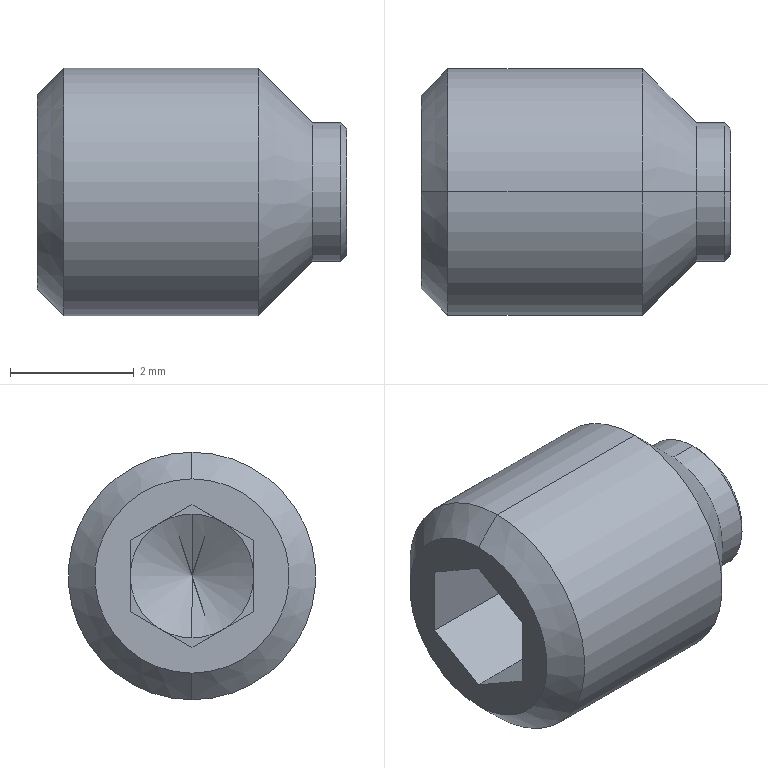Part | NX | features BREP 1 | 1 solid | 26 faces | box 5 x 4 x 4 mm | volume 47.048 mm3 | plane 14 | cone 8 | cylinder 4 | commonest cylinder face diameters 2.25 x2 4 x2